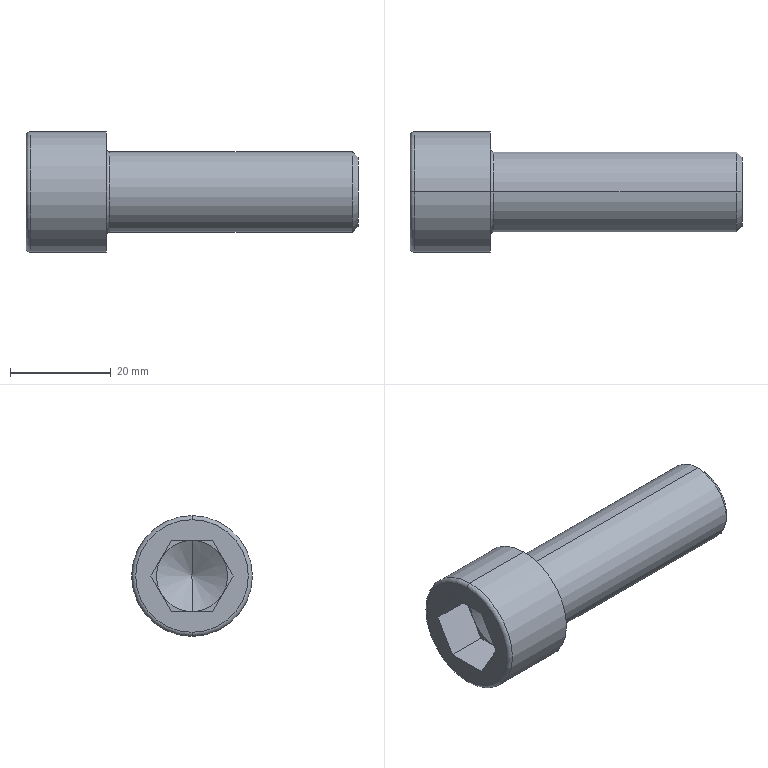Part | STEP file | P-001072_JIS B 1176 M16 x 50 (50) --N | 1 solid | 27 faces | box 66 x 24 x 24 mm | volume 15657 mm3 | plane 15 | cone 4 | torus 4 | cylinder 4 | commonest cylinder face diameters 16 x2 24 x2